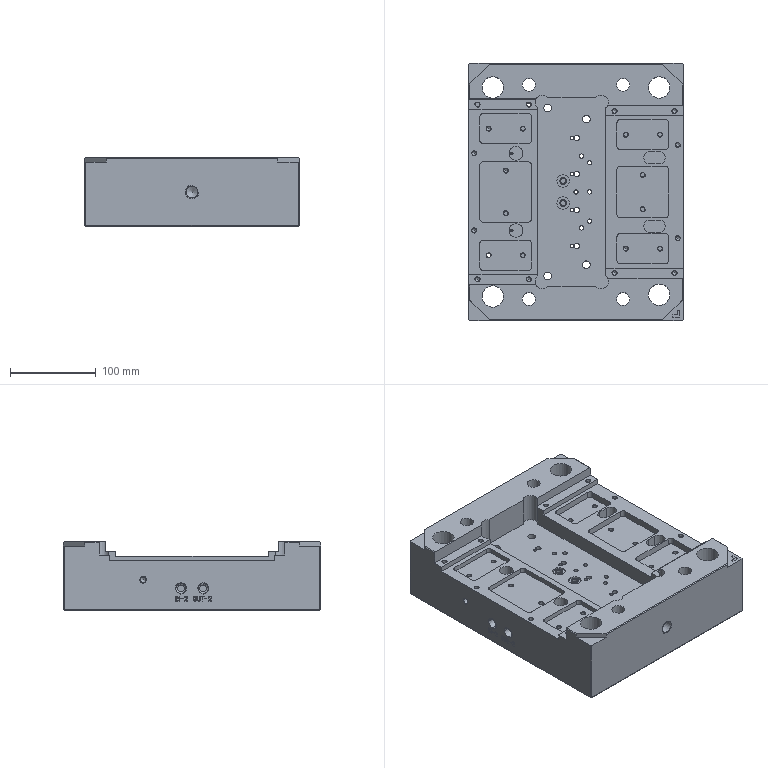NC program | PowerMill | posted with a generic post | part box 250 x 300 x 80 mm
Lines 1 to 829 of 3724:
%
O0001
N104 ( POWERMILL CB  : 2026004.0)
N105 ( POST VER      : 2026.0.0.5161)
N106 ( OPTION FILE   : FANUC)
N107 ( OUTPUT WORKPLANE : 2)
N108 (  )
N109 ( TOOL LIST )
N110 (-------------------------------------)
N111 ( NO. | ID      | DIA.| TIP RAD|LENGTH)
N112 (-------------------------------------)
N113 (    1|B21R0.8_1|21.0 |  0.8   | 89.0 )
N114 (-------------------------------------)
N115 (  )
N116 ( NUMBER OF TOOLPATHS: 1.0 )
N117 ( ESTIMATED PROGRAM DURATION: 0 HOURS 1 MIN 35 SEC)
N118 (  )
N119 G00 G21 G80 G40 G17
N120 G90
N121 G54
N122 G53 Z0.0
N123 (---------------)
N124 ( START TOOLPATH : 05中光-B21R0.8-等高 )
N125 (---------------)
N126 ( TOOL NO.    :1 )
N127 ( TOOL TYPE   : TIPRADIUSED)
N128 ( TOOL ID     : B21R0.8_1)
N129 ( TOOL DIA    : 21.0 LENGTH 89.0)
N130 T1
N131 M6
N132 S2200 M03
N133 G00 G90 X-121.4365 Y-138.4454
N134 G43 Z22.0 H1
N135
N136 G05 P10000 R8
N137 Z2.8
N138 G01 Z-0.2 F2700.0
N139 G03 X-125.6144 Y-134.2235 I-4.2 J0.022 F4500.0
N140 G01 X-126.3455 Y-134.2197
N141 X-126.9934 Y-134.1795
N142 X-127.6413 Y-134.0925
N143 X-128.2892 Y-133.9649
N144 X-128.9147 Y-133.8043
N145 X-129.585 Y-133.5755
N146 X-130.233 Y-133.3081
N147 X-130.5565 Y-133.1564
N148 X-130.8809 Y-132.9857
N149 X-131.5288 Y-132.6023
N150 X-131.6741 Y-132.5085
N151 X-132.1767 Y-132.1527
N152 X-132.5413 Y-131.8606
N153 X-132.8246 Y-131.619
N154 X-133.4725 Y-130.992
N155 X-156.1495 Y-108.3149
N156 X-156.559 Y-107.8878
N157 X-156.7974 Y-107.6162
N158 X-157.1008 Y-107.2399
N159 X-157.5651 Y-106.5919
N160 X-157.9504 Y-105.944
N161 X-158.0932 Y-105.6812
N162 X-158.2817 Y-105.2961
N163 X-158.5562 Y-104.6482
N164 X-158.7411 Y-104.119
N165 X-158.9519 Y-103.3524
N166 X-159.0813 Y-102.7045
N167 X-159.1739 Y-102.0565
N168 X-159.2174 Y-101.4086
N169 X-159.2258 Y-100.2331
N170 G03 X-163.4557 Y-96.0632 I-4.1999 J-0.03
N171 G01 X-163.5518 Y-96.0639
N172 X-163.6056 Y-96.0655 Z-0.2097
N173 X-163.6526 Y-96.0695 Z-0.2374
N174 X-163.7251 Y-96.0781 Z-0.3
N175 X-163.7445 Y-96.0829 Z-0.3375
N176 X-163.7267 Y-96.0884 Z-0.3844
N177 X-163.6872 Y-96.0898 Z-0.4
N178 G02 X-159.4314 Y-100.2331 I0.0562 J-4.1996
N179 G01 X-159.4156 Y-101.4086
N180 X-159.3606 Y-102.0565
N181 X-159.2654 Y-102.7045
N182 X-159.1298 Y-103.3524
N183 X-158.9519 Y-104.0003
N184 X-158.7411 Y-104.6201
N185 X-158.4624 Y-105.2961
N186 X-158.1397 Y-105.944
N187 X-157.7602 Y-106.5919
N188 X-157.4453 Y-107.0536
N189 X-157.3077 Y-107.2399
N190 X-156.7974 Y-107.8686
N191 X-156.1495 Y-108.5473
N192 X-133.4725 Y-131.2243
N193 X-132.8246 Y-131.836
N194 X-132.1767 Y-132.3578
N195 X-131.9663 Y-132.5085
N196 X-131.5288 Y-132.7974
N197 X-130.9153 Y-133.1564
N198 X-130.233 Y-133.4896
N199 X-129.585 Y-133.7539
N200 X-128.9371 Y-133.9709
N201 X-128.2892 Y-134.1447
N202 X-127.6413 Y-134.2765
N203 X-126.9934 Y-134.3677
N204 X-126.3455 Y-134.4189
N205 X-125.6144 Y-134.4314
N206 G02 X-121.4869 Y-138.7026 I-0.0719 J-4.1993
N207 G01 X-121.4887 Y-138.8054
N208 X-121.4919 Y-138.8601 Z-0.4093
N209 X-121.4994 Y-138.9082 Z-0.4361
N210 X-121.5167 Y-138.9872 Z-0.5001
N211 X-121.5259 Y-139.0075 Z-0.5371
N212 X-121.5364 Y-138.9898 Z-0.5843
N213 X-121.5389 Y-138.9496 Z-0.6
N214 G03 X-125.6144 Y-134.6287 I-4.1982 J0.1227
N215 G01 X-126.3455 Y-134.6073
N216 X-126.9934 Y-134.5438
N217 X-127.6413 Y-134.4402
N218 X-128.2892 Y-134.2959
N219 X-128.9371 Y-134.1092
N220 X-129.585 Y-133.8791
N221 X-130.233 Y-133.6025
N222 X-130.8809 Y-133.277
N223 X-131.0974 Y-133.1564
N224 X-131.5288 Y-132.8981
N225 X-132.1767 Y-132.4574
N226 X-132.9203 Y-131.8606
N227 X-133.4725 Y-131.3403
N228 X-156.2747 Y-108.5357
N229 X-156.7974 Y-107.9924
N230 X-157.4123 Y-107.2399
N231 X-157.8571 Y-106.5919
N232 X-158.0932 Y-106.2066
N233 X-158.2425 Y-105.944
N234 X-158.5729 Y-105.2961
N235 X-158.7411 Y-104.9219
N236 X-158.854 Y-104.6482
N237 X-159.0888 Y-104.0003
N238 X-159.2794 Y-103.3524
N239 X-159.428 Y-102.7045
N240 X-159.5355 Y-102.0565
N241 X-159.6029 Y-101.4086
N242 X-159.6305 Y-100.7607
N243 X-159.6314 Y-100.2331
N244 G03 X-163.8382 Y-96.0399 I-4.2 J-0.0068
N245 G01 X-163.9353 Y-96.0401
N246 X-163.9895 Y-96.0419 Z-0.6096
N247 X-164.0368 Y-96.0469 Z-0.6373
N248 X-164.1104 Y-96.0582 Z-0.7
N249 X-164.13 Y-96.0647 Z-0.7375
N250 X-164.1122 Y-96.0724 Z-0.7844
N251 X-164.0725 Y-96.0746 Z-0.8
N252 G02 X-159.8314 Y-100.2331 I0.0413 J-4.1998
N253 G01 X-159.8262 Y-100.7607
N254 X-159.7864 Y-101.4086
N255 X-159.7066 Y-102.0565
N256 X-159.5865 Y-102.7045
N257 X-159.4251 Y-103.3524
N258 X-159.2211 Y-104.0003
N259 X-158.9723 Y-104.6482
N260 X-158.7411 Y-105.1635
N261 X-158.3298 Y-105.944
N262 X-158.0932 Y-106.3356
N263 X-157.9277 Y-106.5919
N264 X-157.4638 Y-107.2399
N265 X-156.9296 Y-107.8878
N266 X-156.7974 Y-108.0345
N267 X-156.3136 Y-108.5357
N268 X-133.4725 Y-131.3767
N269 X-132.8246 Y-131.985
N270 X-132.1813 Y-132.5085
N271 X-131.5288 Y-132.9693
N272 X-131.2343 Y-133.1564
N273 X-130.8809 Y-133.366
N274 X-130.233 Y-133.7075
N275 X-129.585 Y-133.9986
N276 X-128.9371 Y-134.243
N277 X-128.2892 Y-134.4427
N278 X-127.6413 Y-134.6001
N279 X-126.9934 Y-134.7161
N280 X-126.3455 Y-134.792
N281 X-125.6144 Y-134.8256
N282 G02 X-121.6118 Y-139.2141 I-0.193 J-4.1956
N283 G01 X-121.6173 Y-139.3337
N284 X-121.6237 Y-139.3909 Z-0.8086
N285 X-121.6371 Y-139.4419 Z-0.8336
N286 X-121.6709 Y-139.5365 Z-0.9003
N287 X-121.6872 Y-139.5588 Z-0.9363
N288 X-121.7056 Y-139.5404 Z-0.9841
N289 X-121.7093 Y-139.498 Z-1.0
N290 G03 X-125.6144 Y-135.0226 I-4.1903 J0.2851
N291 G01 X-126.3455 Y-134.9729
N292 X-126.9934 Y-134.8848
N293 X-127.6413 Y-134.7559
N294 X-128.2892 Y-134.5856
N295 X-128.9371 Y-134.3724
N296 X-129.585 Y-134.1139
N297 X-130.2394 Y-133.8043
N298 X-130.8809 Y-133.4496
N299 X-131.5288 Y-133.0351
N300 X-132.2377 Y-132.5085
N301 X-132.8246 Y-132.0066
N302 X-133.4725 Y-131.3767
N303 X-156.3136 Y-108.5357
N304 X-156.9484 Y-107.8878
N305 X-157.5069 Y-107.2399
N306 X-157.9914 Y-106.5919
N307 X-158.4118 Y-105.944
N308 X-158.7749 Y-105.2961
N309 X-159.0863 Y-104.6482
N310 X-159.3891 Y-103.8904
N311 X-159.5669 Y-103.3524
N312 X-159.7411 Y-102.7045
N313 X-159.874 Y-102.0565
N314 X-159.9661 Y-101.4086
N315 X-160.0181 Y-100.7607
N316 X-160.0314 Y-100.2331
N317 G03 X-164.3356 Y-96.14 I-4.1987 J-0.1055
N318 G01 X-164.4504 Y-96.1428
N319 X-164.513 Y-96.1504 Z-1.0095
N320 X-164.5676 Y-96.1689 Z-1.0367
N321 X-164.6549 Y-96.2112 Z-1.1003
N322 X-164.6771 Y-96.2345 Z-1.1373
N323 X-164.656 Y-96.2619 Z-1.1843
N324 X-164.6101 Y-96.2694 Z-1.2
N325 G02 X-160.2277 Y-100.2787 I0.1865 J-4.1958
N326 G01 X-160.2063 Y-100.7607
N327 X-160.1419 Y-101.4086
N328 X-160.037 Y-102.0568
N329 X-159.8919 Y-102.7045
N330 X-159.7044 Y-103.3524
N331 X-159.4731 Y-104.0003
N332 X-159.1953 Y-104.6482
N333 X-158.8687 Y-105.2961
N334 X-158.7411 Y-105.5238
N335 X-158.4884 Y-105.944
N336 X-158.0932 Y-106.5309
N337 X-157.5428 Y-107.2399
N338 X-156.9591 Y-107.8878
N339 X-156.7974 Y-108.0518
N340 X-132.9885 Y-131.8606
N341 X-132.8246 Y-132.0199
N342 X-132.2807 Y-132.5085
N343 X-131.5288 Y-133.0948
N344 X-130.8809 Y-133.528
N345 X-130.233 Y-133.9029
N346 X-129.585 Y-134.2245
N347 X-129.0527 Y-134.4522
N348 X-128.2892 Y-134.7246
N349 X-127.6413 Y-134.9079
N350 X-126.9934 Y-135.0494
N351 X-126.3455 Y-135.1499
N352 X-125.623 Y-135.215
N353 G02 X-121.8167 Y-139.7748 I-0.3768 J-4.183
N354 G01 X-121.8236 Y-139.8517
N355 X-121.8303 Y-139.9066 Z-1.2114
N356 X-121.8393 Y-139.9518 Z-1.2438
N357 X-121.8524 Y-140.0033 Z-1.3
N358 X-121.8596 Y-140.0187 Z-1.3394
N359 X-121.8642 Y-139.998 Z-1.3849
N360 X-121.8625 Y-139.9579 Z-1.4
N361 G03 X-125.635 Y-135.3702 I-4.1802 J0.4076
N362 G01 X-126.3455 Y-135.3009
N363 X-126.9934 Y-135.1994
N364 X-127.4447 Y-135.1001
N365 X-127.6413 Y-135.0487
N366 X-128.2892 Y-134.8564
N367 X-128.9371 Y-134.6177
N368 X-129.3238 Y-134.4522
N369 X-129.585 Y-134.3307
N370 X-130.233 Y-133.9929
N371 X-130.5566 Y-133.8043
N372 X-130.8809 Y-133.6008
N373 X-131.5288 Y-133.1481
N374 X-132.1767 Y-132.6263
N375 X-132.3115 Y-132.5085
N376 X-132.8246 Y-132.0246
N377 X-156.9615 Y-107.8878
N378 X-157.4453 Y-107.3819
N379 X-157.5717 Y-107.2399
N380 X-158.1004 Y-106.5919
N381 X-158.5595 Y-105.944
N382 X-158.7411 Y-105.6594
N383 X-158.9572 Y-105.2961
N384 X-159.3001 Y-104.6482
N385 X-159.5908 Y-104.0003
N386 X-159.8344 Y-103.3524
N387 X-160.037 Y-102.6953
N388 X-160.1863 Y-102.0565
N389 X-160.2927 Y-101.4086
N390 X-160.3639 Y-100.7607
N391 X-160.3841 Y-100.3209
N392 G03 X-164.7726 Y-96.3182 I-4.1956 J-0.1929
N393 G01 X-164.8168 Y-96.3202
N394 X-164.877 Y-96.3271 Z-1.4166
N395 X-164.9189 Y-96.3403 Z-1.4616
N396 X-164.9384 Y-96.3507 Z-1.5
N397 X-164.9443 Y-96.3617 Z-1.5437
N398 X-164.917 Y-96.3708 Z-1.5859
N399 X-164.8739 Y-96.3721 Z-1.6
N400 G02 X-160.4669 Y-100.3544 I0.2123 J-4.1946
N401 G01 X-160.4464 Y-100.7607
N402 X-160.3763 Y-101.4086
N403 X-160.2703 Y-102.0565
N404 X-160.1185 Y-102.7045
N405 X-160.037 Y-102.994
N406 X-159.9227 Y-103.3524
N407 X-159.68 Y-104.0003
N408 X-159.3861 Y-104.6482
N409 X-159.0356 Y-105.2961
N410 X-158.7411 Y-105.7699
N411 X-158.6233 Y-105.944
N412 X-158.1451 Y-106.5919
N413 X-157.5926 Y-107.2399
N414 X-156.9615 Y-107.8878
N415 X-132.8246 Y-132.0246
N416 X-132.1767 Y-132.65
N417 X-131.5775 Y-133.1564
N418 X-130.8809 Y-133.6675
N419 X-130.6718 Y-133.8043
N420 X-130.233 Y-134.07
N421 X-129.585 Y-134.4164
N422 X-128.9371 Y-134.7028
N423 X-128.2892 Y-134.9413
N424 X-127.7717 Y-135.1001
N425 X-126.9934 Y-135.2822
N426 X-126.3455 Y-135.3866
N427 X-125.643 Y-135.4539
N428 G02 X-121.863 Y-140.0356 I-0.4008 J-4.1809
N429 G01 X-121.8633 Y-140.039
N430 X-121.8678 Y-140.1086 Z-1.6281
N431 X-121.8656 Y-140.1395 Z-1.6966
N432 X-121.8653 Y-140.1397 Z-1.7
N433 X-121.8576 Y-140.1131 Z-1.7705
N434 X-121.849 Y-140.0439 Z-1.8
N435 G03 X-125.6473 Y-135.4775 I-4.1824 J0.384
N436 G01 X-126.3455 Y-135.4134
N437 X-126.9934 Y-135.309
N438 X-127.6413 Y-135.1623
N439 X-128.2892 Y-134.9715
N440 X-128.9371 Y-134.7339
N441 X-129.585 Y-134.446
N442 X-130.233 Y-134.1031
N443 X-130.7214 Y-133.8043
N444 X-130.8809 Y-133.6986
N445 X-131.6124 Y-133.1564
N446 X-132.1767 Y-132.6645
N447 X-132.3398 Y-132.5085
N448 X-157.4453 Y-107.4038
N449 X-157.6049 Y-107.2399
N450 X-158.1729 Y-106.5919
N451 X-158.6555 Y-105.944
N452 X-159.0665 Y-105.2961
N453 X-159.4151 Y-104.6482
N454 X-159.7081 Y-104.0003
N455 X-159.9504 Y-103.3524
N456 X-160.037 Y-103.0837
N457 X-160.1457 Y-102.7045
N458 X-160.2966 Y-102.0565
N459 X-160.405 Y-101.4086
N460 X-160.4724 Y-100.7607
N461 X-160.4912 Y-100.3808
N462 G03 X-164.8933 Y-96.3932 I-4.1948 J-0.2073
N463 G01 X-164.9064 Y-96.3939
N464 X-164.9744 Y-96.4035 Z-1.8249
N465 X-165.0082 Y-96.4208 Z-1.8873
N466 X-165.0099 Y-96.4241 Z-1.9001
N467 X-164.9874 Y-96.4403 Z-1.9699
N468 X-164.9187 Y-96.4441 Z-2.0
N469 G02 X-160.4922 Y-100.4046 I0.233 J-4.1935
N470 G01 X-160.4724 Y-100.7607
N471 X-160.405 Y-101.4086
N472 X-160.2966 Y-102.0565
N473 X-160.1457 Y-102.7045
N474 X-160.037 Y-103.0837
N475 X-159.9504 Y-103.3524
N476 X-159.7081 Y-104.0003
N477 X-159.4151 Y-104.6482
N478 X-159.0665 Y-105.2961
N479 X-158.6555 Y-105.944
N480 X-158.1729 Y-106.5919
N481 X-157.6049 Y-107.2399
N482 X-157.4453 Y-107.4038
N483 X-132.3398 Y-132.5085
N484 X-132.1767 Y-132.6645
N485 X-131.6124 Y-133.1564
N486 X-130.8809 Y-133.6986
N487 X-130.7214 Y-133.8043
N488 X-130.233 Y-134.1031
N489 X-129.585 Y-134.446
N490 X-128.9371 Y-134.7339
N491 X-128.2892 Y-134.9715
N492 X-127.6413 Y-135.1623
N493 X-126.9934 Y-135.309
N494 X-126.3455 Y-135.4134
N495 X-125.6505 Y-135.4798
N496 G02 X-121.8691 Y-140.0604 I-0.3996 J-4.181
N497 G01 X-121.8692 Y-140.0607
N498 X-121.8764 Y-140.1309 Z-2.0292
N499 X-121.8805 Y-140.1601 Z-2.0997
N500 Z-2.1
N501 X-121.8789 Y-140.131 Z-2.1707
N502 X-121.8727 Y-140.0607 Z-2.2
N503 G03 X-125.6535 Y-135.4796 I-4.1809 J0.4002
N504 G01 X-126.3455 Y-135.4134
N505 X-126.9934 Y-135.309
N506 X-127.6413 Y-135.1623
N507 X-128.2892 Y-134.9715
N508 X-128.9371 Y-134.7339
N509 X-129.585 Y-134.446
N510 X-130.233 Y-134.1031
N511 X-130.7214 Y-133.8043
N512 X-130.8809 Y-133.6986
N513 X-131.6124 Y-133.1564
N514 X-132.1767 Y-132.6645
N515 X-132.3398 Y-132.5085
N516 X-157.4453 Y-107.4039
N517 X-157.6049 Y-107.2399
N518 X-158.1729 Y-106.5919
N519 X-158.6555 Y-105.944
N520 X-159.0665 Y-105.2961
N521 X-159.4151 Y-104.6482
N522 X-159.7081 Y-104.0003
N523 X-159.9504 Y-103.3524
N524 X-160.037 Y-103.0837
N525 X-160.1457 Y-102.7045
N526 X-160.2966 Y-102.0565
N527 X-160.405 Y-101.4086
N528 X-160.4724 Y-100.7607
N529 X-160.4913 Y-100.4281
N530 G03 X-164.9223 Y-96.4725 I-4.1932 J-0.2377
N531 G01 X-164.9402 Y-96.4736
N532 X-165.0078 Y-96.4849 Z-2.2235
N533 X-165.0434 Y-96.5058 Z-2.283
N534 X-165.0464 Y-96.5115 Z-2.3001
N535 X-165.0262 Y-96.5321 Z-2.3695
N536 X-164.9577 Y-96.5372 Z-2.4
N537 G02 X-160.4903 Y-100.4515 I0.2765 J-4.1909
N538 G01 X-160.4586 Y-100.9311
N539 X-160.4051 Y-101.4086
N540 X-160.2966 Y-102.0565
N541 X-160.1457 Y-102.7045
N542 X-160.037 Y-103.0837
N543 X-159.9504 Y-103.3524
N544 X-159.7081 Y-104.0003
N545 X-159.4151 Y-104.6482
N546 X-159.0665 Y-105.2961
N547 X-158.6555 Y-105.944
N548 X-158.1729 Y-106.5919
N549 X-157.6049 Y-107.2399
N550 X-157.4453 Y-107.4039
N551 X-132.3398 Y-132.5085
N552 X-132.1767 Y-132.6645
N553 X-131.6124 Y-133.1564
N554 X-130.8809 Y-133.6986
N555 X-130.7214 Y-133.8043
N556 X-130.233 Y-134.1031
N557 X-129.585 Y-134.446
N558 X-128.9371 Y-134.7339
N559 X-128.2892 Y-134.9715
N560 X-127.6413 Y-135.1624
N561 X-126.9934 Y-135.309
N562 X-126.3455 Y-135.4134
N563 X-125.6565 Y-135.4794
N564 G02 X-121.8763 Y-140.061 I-0.4007 J-4.1809
N565 G01 X-121.8764 Y-140.0613
N566 X-121.8836 Y-140.1315 Z-2.4292
N567 X-121.8877 Y-140.1607 Z-2.4996
N568 Z-2.5
N569 X-121.8863 Y-140.1317 Z-2.5707
N570 X-121.88 Y-140.0614 Z-2.6
N571 G03 X-125.6595 Y-135.4793 I-4.1808 J0.4014
N572 G01 X-126.3455 Y-135.4134
N573 X-126.9934 Y-135.309
N574 X-127.6413 Y-135.1624
N575 X-128.2892 Y-134.9715
N576 X-128.9371 Y-134.7339
N577 X-129.585 Y-134.446
N578 X-130.233 Y-134.1031
N579 X-130.7214 Y-133.8043
N580 X-130.8809 Y-133.6986
N581 X-131.6124 Y-133.1564
N582 X-132.1767 Y-132.6645
N583 X-132.3398 Y-132.5085
N584 X-157.4453 Y-107.4039
N585 X-157.6049 Y-107.2399
N586 X-158.1729 Y-106.5919
N587 X-158.6556 Y-105.944
N588 X-159.0665 Y-105.2961
N589 X-159.4151 Y-104.6482
N590 X-159.7081 Y-104.0003
N591 X-159.9504 Y-103.3524
N592 X-160.037 Y-103.0837
N593 X-160.1457 Y-102.7045
N594 X-160.2966 Y-102.0565
N595 X-160.4051 Y-101.4086
N596 X-160.4576 Y-100.9428
N597 X-160.4893 Y-100.475
N598 G03 X-164.9633 Y-96.5683 I-4.1904 J-0.2837
N599 G01 X-165.0054 Y-96.5711
N600 X-165.0752 Y-96.5873 Z-2.6181
N601 X-165.1199 Y-96.6209 Z-2.6665
N602 X-165.1351 Y-96.6435 Z-2.7006
N603 X-165.1372 Y-96.6712 Z-2.7448
N604 X-165.1028 Y-96.6938 Z-2.7862
N605 X-165.0527 Y-96.6978 Z-2.8
N606 G02 X-160.4882 Y-100.4985 I0.3819 J-4.1826
N607 G01 X-160.4051 Y-101.4086
N608 X-160.2966 Y-102.0565
N609 X-160.1457 Y-102.7045
N610 X-160.037 Y-103.0837
N611 X-159.9504 Y-103.3524
N612 X-159.7081 Y-104.0003
N613 X-159.4151 Y-104.6482
N614 X-159.0665 Y-105.2961
N615 X-158.6556 Y-105.944
N616 X-158.1729 Y-106.5919
N617 X-157.6049 Y-107.2399
N618 X-157.4453 Y-107.4039
N619 X-132.3398 Y-132.5085
N620 X-132.1767 Y-132.6645
N621 X-131.6124 Y-133.1564
N622 X-130.8809 Y-133.6986
N623 X-130.7214 Y-133.8043
N624 X-130.233 Y-134.1031
N625 X-129.585 Y-134.446
N626 X-128.9371 Y-134.7339
N627 X-128.2892 Y-134.9715
N628 X-127.6413 Y-135.1624
N629 X-126.9934 Y-135.309
N630 X-126.3455 Y-135.4134
N631 X-125.6625 Y-135.4791
N632 G02 X-121.8838 Y-140.0618 I-0.402 J-4.1807
N633 G01 Y-140.0621
N634 X-121.8911 Y-140.1323 Z-2.8292
N635 X-121.8951 Y-140.1615 Z-2.8997
N636 Z-2.9
N637 X-121.8936 Y-140.1324 Z-2.9707
N638 X-121.8874 Y-140.062 Z-3.0
N639 G03 X-125.6655 Y-135.4789 I-4.1806 J0.4024
N640 G01 X-126.3455 Y-135.4134
N641 X-126.9934 Y-135.309
N642 X-127.6413 Y-135.1624
N643 X-128.2892 Y-134.9715
N644 X-128.9371 Y-134.7339
N645 X-129.585 Y-134.446
N646 X-130.233 Y-134.1031
N647 X-130.7214 Y-133.8043
N648 X-130.8809 Y-133.6986
N649 X-131.6124 Y-133.1564
N650 X-132.1767 Y-132.6645
N651 X-132.3398 Y-132.5085
N652 X-157.4453 Y-107.4039
N653 X-157.6049 Y-107.2399
N654 X-158.1729 Y-106.5919
N655 X-158.6556 Y-105.944
N656 X-159.0665 Y-105.2961
N657 X-159.4151 Y-104.6482
N658 X-159.7081 Y-104.0003
N659 X-159.9504 Y-103.3524
N660 X-160.037 Y-103.0837
N661 X-160.1457 Y-102.7045
N662 X-160.2966 Y-102.0565
N663 X-160.4051 Y-101.4086
N664 X-160.487 Y-100.522
N665 G03 X-165.0558 Y-96.7263 I-4.1822 J-0.3865
N666 G01 X-165.0585 Y-96.7266
N667 X-165.1283 Y-96.7371 Z-3.0283
N668 X-165.1578 Y-96.7496 Z-3.0972
N669 X-165.1579 Y-96.75 Z-3.1
N670 X-165.1293 Y-96.7574 Z-3.1705
N671 X-165.0588 Y-96.755 Z-3.2
N672 G02 X-160.4858 Y-100.5454 I0.3912 J-4.1817
N673 G01 X-160.4051 Y-101.4086
N674 X-160.2966 Y-102.0565
N675 X-160.1457 Y-102.7045
N676 X-160.037 Y-103.0837
N677 X-159.9504 Y-103.3524
N678 X-159.7081 Y-104.0003
N679 X-159.4151 Y-104.6482
N680 X-159.0665 Y-105.2961
N681 X-158.6556 Y-105.944
N682 X-158.1729 Y-106.5919
N683 X-157.6049 Y-107.2399
N684 X-157.4453 Y-107.4039
N685 X-132.3398 Y-132.5085
N686 X-132.1767 Y-132.6645
N687 X-131.6124 Y-133.1564
N688 X-130.8809 Y-133.6986
N689 X-130.7214 Y-133.8043
N690 X-130.233 Y-134.1031
N691 X-129.585 Y-134.446
N692 X-128.9371 Y-134.7339
N693 X-128.2892 Y-134.9715
N694 X-127.6413 Y-135.1624
N695 X-126.9934 Y-135.309
N696 X-126.3455 Y-135.4134
N697 X-125.6686 Y-135.4787
N698 G02 X-121.891 Y-140.0624 I-0.403 J-4.1806
N699 G01 Y-140.0627
N700 X-121.8983 Y-140.1329 Z-3.2292
N701 X-121.9024 Y-140.1621 Z-3.2997
N702 Z-3.3
N703 X-121.9009 Y-140.133 Z-3.3707
N704 X-121.8946 Y-140.0627 Z-3.4
N705 G03 X-125.6716 Y-135.4785 I-4.1806 J0.4036
N706 G01 X-126.3455 Y-135.4134
N707 X-126.9934 Y-135.3091
N708 X-127.6413 Y-135.1624
N709 X-128.2892 Y-134.9715
N710 X-128.9371 Y-134.7339
N711 X-129.585 Y-134.446
N712 X-130.233 Y-134.1031
N713 X-130.7214 Y-133.8043
N714 X-130.8809 Y-133.6986
N715 X-131.6124 Y-133.1564
N716 X-132.1767 Y-132.6645
N717 X-132.3398 Y-132.5085
N718 X-157.4453 Y-107.4039
N719 X-157.6049 Y-107.2399
N720 X-158.1729 Y-106.5919
N721 X-158.6556 Y-105.944
N722 X-159.0665 Y-105.2961
N723 X-159.4151 Y-104.6482
N724 X-159.7081 Y-104.0003
N725 X-159.9504 Y-103.3524
N726 X-160.037 Y-103.0837
N727 X-160.1457 Y-102.7045
N728 X-160.2966 Y-102.0565
N729 X-160.4051 Y-101.4086
N730 X-160.4846 Y-100.5689
N731 G03 X-165.0617 Y-96.7834 I-4.1813 J-0.3958
N732 G01 X-165.0645 Y-96.7837
N733 X-165.1342 Y-96.7943 Z-3.4283
N734 X-165.1637 Y-96.8069 Z-3.4972
N735 X-165.1638 Y-96.8073 Z-3.5
N736 X-165.1352 Y-96.8146 Z-3.5705
N737 X-165.0647 Y-96.812 Z-3.6
N738 G02 X-160.4833 Y-100.5923 I0.4006 J-4.1808
N739 G01 X-160.4051 Y-101.4086
N740 X-160.2966 Y-102.0565
N741 X-160.1457 Y-102.7045
N742 X-160.037 Y-103.0837
N743 X-159.9504 Y-103.3524
N744 X-159.7081 Y-104.0003
N745 X-159.4151 Y-104.6482
N746 X-159.0665 Y-105.2961
N747 X-158.6556 Y-105.944
N748 X-158.1729 Y-106.5919
N749 X-157.6049 Y-107.2399
N750 X-157.4453 Y-107.4039
N751 X-132.3398 Y-132.5085
N752 X-132.1767 Y-132.6645
N753 X-131.6124 Y-133.1564
N754 X-130.8809 Y-133.6986
N755 X-130.7214 Y-133.8043
N756 X-130.233 Y-134.1031
N757 X-129.585 Y-134.446
N758 X-128.9371 Y-134.7339
N759 X-128.2892 Y-134.9715
N760 X-127.6413 Y-135.1624
N761 X-126.9934 Y-135.3091
N762 X-126.3455 Y-135.4134
N763 X-125.6746 Y-135.4783
N764 G02 X-121.8982 Y-140.063 I-0.4042 J-4.1805
N765 G01 X-121.8983 Y-140.0633
N766 X-121.9056 Y-140.1336 Z-3.6292
N767 X-121.9097 Y-140.1627 Z-3.6997
N768 Z-3.7
N769 X-121.9082 Y-140.1336 Z-3.7707
N770 X-121.9019 Y-140.0633 Z-3.8
N771 G03 X-125.6776 Y-135.4781 I-4.1804 J0.4047
N772 G01 X-126.3455 Y-135.4134
N773 X-126.9934 Y-135.3091
N774 X-127.6413 Y-135.1624
N775 X-128.2892 Y-134.9715
N776 X-128.9371 Y-134.7339
N777 X-129.585 Y-134.446
N778 X-130.233 Y-134.1031
N779 X-130.7214 Y-133.8043
N780 X-130.8809 Y-133.6986
N781 X-131.6124 Y-133.1564
N782 X-132.1767 Y-132.6645
N783 X-132.3398 Y-132.5085
N784 X-157.4453 Y-107.4039
N785 X-157.6049 Y-107.2399
N786 X-158.1729 Y-106.5919
N787 X-158.6556 Y-105.944
N788 X-159.0665 Y-105.2961
N789 X-159.4151 Y-104.6482
N790 X-159.7081 Y-104.0003
N791 X-159.9504 Y-103.3524
N792 X-160.037 Y-103.0837
N793 X-160.1457 Y-102.7045
N794 X-160.2966 Y-102.0565
N795 X-160.4051 Y-101.4086
N796 X-160.4819 Y-100.6158
N797 G03 X-165.0675 Y-96.8405 I-4.1804 J-0.4051
N798 G01 X-165.0702 Y-96.8408
N799 X-165.14 Y-96.8516 Z-3.8283
N800 X-165.1694 Y-96.8642 Z-3.8973
N801 Y-96.8646 Z-3.9
N802 X-165.1408 Y-96.8718 Z-3.9705
N803 X-165.0703 Y-96.8691 Z-4.0
N804 G02 X-160.4805 Y-100.6392 I0.4098 J-4.1799
N805 G01 X-160.4051 Y-101.4086
N806 X-160.2966 Y-102.0565
N807 X-160.1457 Y-102.7045
N808 X-160.037 Y-103.0837
N809 X-159.9504 Y-103.3524
N810 X-159.7081 Y-104.0003
N811 X-159.4151 Y-104.6482
N812 X-159.0665 Y-105.2961
N813 X-158.6556 Y-105.944
N814 X-158.1729 Y-106.5919
N815 X-157.6049 Y-107.2399
N816 X-157.4453 Y-107.4039
N817 X-132.3398 Y-132.5085
N818 X-132.1767 Y-132.6645
N819 X-131.6124 Y-133.1564
N820 X-130.8809 Y-133.6986
N821 X-130.7214 Y-133.8043
N822 X-130.233 Y-134.1031
N823 X-129.585 Y-134.446
N824 X-128.9371 Y-134.7339
N825 X-128.2892 Y-134.9715
N826 X-127.6413 Y-135.1624
N827 X-126.9934 Y-135.3091
N828 X-126.3455 Y-135.4134
N829 X-125.6806 Y-135.4779
N830 G02 X-121.9056 Y-140.0637 I-0.4054 J-4.1804
N831 G01 X-121.9057 Y-140.0641
N832 X-121.913 Y-140.1343 Z-4.0292
N833 X-121.9171 Y-140.1635 Z-4.0997
N834 Z-4.1
N835 X-121.9156 Y-140.1344 Z-4.1707
N836 X-121.9093 Y-140.0641 Z-4.2
N837 G03 X-125.6836 Y-135.4777 I-4.1803 J0.4061
N838 G01 X-126.3455 Y-135.4134
N839 X-126.9934 Y-135.3091
N840 X-127.6413 Y-135.1624
N841 X-128.2892 Y-134.9715
N842 X-128.9371 Y-134.7339
N843 X-129.585 Y-134.446
N844 X-130.233 Y-134.1031
N845 X-130.7214 Y-133.8043
N846 X-130.8809 Y-133.6986
N847 X-131.6124 Y-133.1564
N848 X-132.1767 Y-132.6646
N849 X-132.3398 Y-132.5085
N850 X-157.4453 Y-107.4039
N851 X-157.6049 Y-107.2399
N852 X-158.1729 Y-106.5919
N853 X-158.6556 Y-105.944
N854 X-159.0665 Y-105.2961
N855 X-159.4151 Y-104.6482
N856 X-159.7082 Y-104.0003
N857 X-159.9505 Y-103.3524
N858 X-160.037 Y-103.0837
N859 X-160.1457 Y-102.7045
N860 X-160.2966 Y-102.0565
N861 X-160.4051 Y-101.4086
N862 X-160.4791 Y-100.6626
N863 G03 X-165.0731 Y-96.8977 I-4.1794 J-0.4145
N864 G01 X-165.0758 Y-96.8979
N865 X-165.1455 Y-96.9089 Z-4.2283
N866 X-165.1749 Y-96.9216 Z-4.2973
N867 X-165.175 Y-96.922 Z-4.3
N868 X-165.1463 Y-96.9291 Z-4.3705
N869 X-165.0758 Y-96.9262 Z-4.4
N870 G02 X-160.4776 Y-100.6861 I0.4192 J-4.179
N871 G01 X-160.4051 Y-101.4086
N872 X-160.2966 Y-102.0565
N873 X-160.1457 Y-102.7045
N874 X-160.037 Y-103.0837
N875 X-159.9505 Y-103.3524
N876 X-159.7082 Y-104.0003
N877 X-159.4151 Y-104.6482
N878 X-159.0665 Y-105.2961
N879 X-158.6556 Y-105.944
N880 X-158.1729 Y-106.5919
N881 X-157.6049 Y-107.2399
N882 X-157.4453 Y-107.4039
N883 X-132.3398 Y-132.5085
N884 X-132.1767 Y-132.6646
N885 X-131.6124 Y-133.1564
N886 X-130.8809 Y-133.6986
N887 X-130.7214 Y-133.8043
N888 X-130.233 Y-134.1031
N889 X-129.585 Y-134.446
N890 X-128.9371 Y-134.7339
N891 X-128.2892 Y-134.9715
N892 X-127.6413 Y-135.1624
N893 X-126.9934 Y-135.3091
N894 X-126.3455 Y-135.4134
N895 X-125.6866 Y-135.4775
N896 G02 X-121.9129 Y-140.0644 I-0.4066 J-4.1803
N897 G01 X-121.913 Y-140.0647
N898 X-121.9203 Y-140.1349 Z-4.4292
N899 X-121.9244 Y-140.1641 Z-4.4997
N900 Z-4.5
N901 X-121.9228 Y-140.135 Z-4.5707
N902 X-121.9165 Y-140.0647 Z-4.6
N903 G03 X-125.6896 Y-135.4773 I-4.1802 J0.4072
N904 G01 X-126.3455 Y-135.4135
N905 X-126.9934 Y-135.3091
N906 X-127.6413 Y-135.1624
N907 X-128.2892 Y-134.9715
N908 X-128.9371 Y-134.7339
N909 X-129.585 Y-134.4461
N910 X-130.233 Y-134.1031
N911 X-130.7214 Y-133.8043
N912 X-130.8809 Y-133.6986
N913 X-131.6124 Y-133.1564
N914 X-132.1767 Y-132.6646
N915 X-132.3398 Y-132.5085
N916 X-157.4453 Y-107.4039
N917 X-157.6049 Y-107.2399
N918 X-158.1729 Y-106.5919
N919 X-158.6556 Y-105.944
N920 X-159.0665 Y-105.2961
N921 X-159.4151 Y-104.6482
N922 X-159.7082 Y-104.0003
N923 X-159.9505 Y-103.3524
N924 X-160.037 Y-103.0837
N925 X-160.1458 Y-102.7045
N926 X-160.2967 Y-102.0565